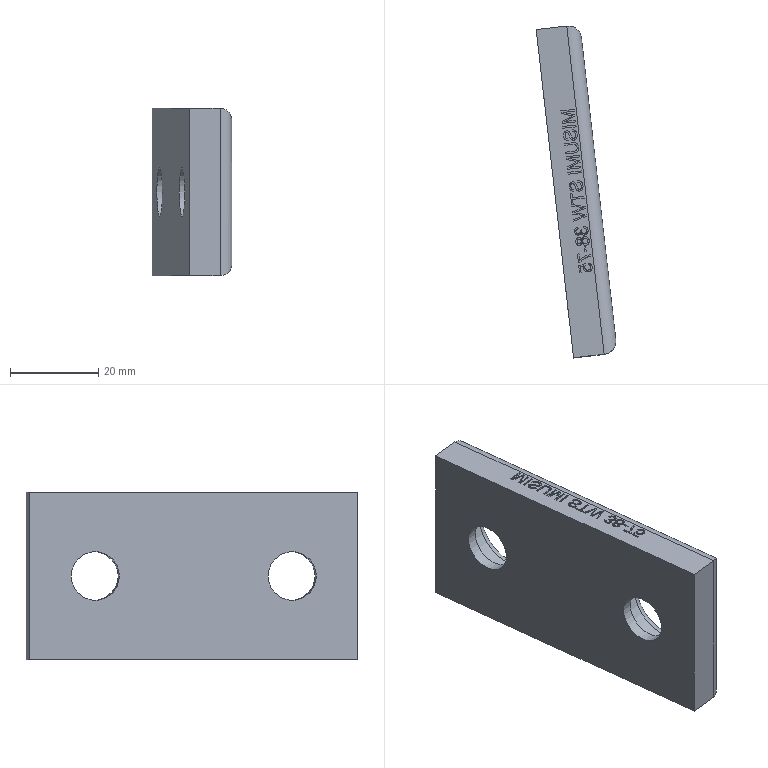Part | NX | features DB 2 | 1 solid | 142 faces | box 18.106 x 75.33 x 38 mm | volume 23885 mm3 | plane 95 | spline 37 | cylinder 8 | torus 2 | commonest cylinder face diameters 6 x4 11 x2 17.5 x2